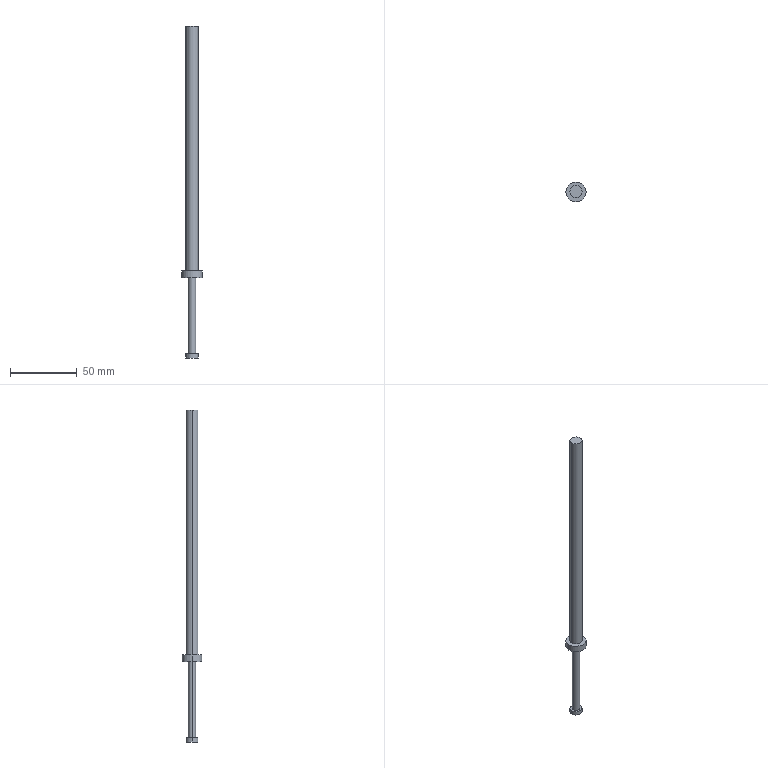Part | Creo | 1 solid | 13 faces | box 15 x 15 x 248 mm | volume 14071 mm3 | cylinder 8 | plane 5 | commonest cylinder face diameters 9 x4 5.5 x2 15 x2
STEP:
#1=CARTESIAN_POINT('',(-188.734,-198.792,-47.5));
#2=VERTEX_POINT('',#1);
#3=CARTESIAN_POINT('',(-179.734,-198.792,-47.5));
#4=VERTEX_POINT('',#3);
#5=CARTESIAN_POINT('',(-184.234,-198.792,-47.5));
#6=DIRECTION('',(0.,0.,1.));
#7=DIRECTION('',(-1.,0.,0.));
#8=AXIS2_PLACEMENT_3D('',#5,#6,#7);
#9=CIRCLE('',#8,4.5);
#10=EDGE_CURVE('',#2,#4,#9,.T.);
#11=ORIENTED_EDGE('',*,*,#10,.T.);
#12=CARTESIAN_POINT('',(-179.734,-198.792,-230.5));
#13=VERTEX_POINT('',#12);
#14=CARTESIAN_POINT('',(-179.734,-198.792,-47.5));
#15=DIRECTION('',(0.,0.,-1.));
#16=VECTOR('',#15,183.);
#17=LINE('',#14,#16);
#18=EDGE_CURVE('',#4,#13,#17,.T.);
#19=ORIENTED_EDGE('',*,*,#18,.T.);
#20=CARTESIAN_POINT('',(-188.734,-198.792,-230.5));
#21=VERTEX_POINT('',#20);
#22=CARTESIAN_POINT('',(-184.234,-198.792,-230.5));
#23=DIRECTION('',(0.,0.,-1.));
#24=DIRECTION('',(1.,0.,0.));
#25=AXIS2_PLACEMENT_3D('',#22,#23,#24);
#26=CIRCLE('',#25,4.5);
#27=EDGE_CURVE('',#13,#21,#26,.T.);
#28=ORIENTED_EDGE('',*,*,#27,.T.);
#29=CARTESIAN_POINT('',(-188.734,-198.792,-47.5));
#30=DIRECTION('',(0.,0.,-1.));
#31=VECTOR('',#30,183.);
#32=LINE('',#29,#31);
#33=EDGE_CURVE('',#2,#21,#32,.T.);
#34=ORIENTED_EDGE('',*,*,#33,.F.);
#35=EDGE_LOOP('',(#11,#19,#28,#34));
#36=FACE_OUTER_BOUND('',#35,.F.);
#37=CARTESIAN_POINT('',(-184.234,-198.792,7.391));
#38=DIRECTION('',(0.,0.,-1.));
#39=DIRECTION('',(1.,0.,0.));
#40=AXIS2_PLACEMENT_3D('',#37,#38,#39);
#41=CYLINDRICAL_SURFACE('',#40,4.5);
#42=ADVANCED_FACE('',(#36),#41,.T.);
#43=ORIENTED_EDGE('',*,*,#10,.F.);
#44=CARTESIAN_POINT('',(-184.234,-198.792,-47.5));
#45=DIRECTION('',(0.,0.,1.));
#46=DIRECTION('',(1.,0.,0.));
#47=AXIS2_PLACEMENT_3D('',#44,#45,#46);
#48=CIRCLE('',#47,4.5);
#49=EDGE_CURVE('',#4,#2,#48,.T.);
#50=ORIENTED_EDGE('',*,*,#49,.F.);
#51=EDGE_LOOP('',(#43,#50));
#52=FACE_OUTER_BOUND('',#51,.F.);
#53=CARTESIAN_POINT('',(0.,0.,-47.5));
#54=DIRECTION('',(0.,0.,-1.));
#55=DIRECTION('',(-1.,0.,0.));
#56=AXIS2_PLACEMENT_3D('',#53,#54,#55);
#57=PLANE('',#56);
#58=ADVANCED_FACE('',(#52),#57,.F.);
#59=ORIENTED_EDGE('',*,*,#49,.T.);
#60=ORIENTED_EDGE('',*,*,#33,.T.);
#61=CARTESIAN_POINT('',(-184.234,-198.792,-230.5));
#62=DIRECTION('',(0.,0.,-1.));
#63=DIRECTION('',(-1.,0.,0.));
#64=AXIS2_PLACEMENT_3D('',#61,#62,#63);
#65=CIRCLE('',#64,4.5);
#66=EDGE_CURVE('',#21,#13,#65,.T.);
#67=ORIENTED_EDGE('',*,*,#66,.T.);
#68=ORIENTED_EDGE('',*,*,#18,.F.);
#69=EDGE_LOOP('',(#59,#60,#67,#68));
#70=FACE_OUTER_BOUND('',#69,.F.);
#71=CARTESIAN_POINT('',(-184.234,-198.792,7.391));
#72=DIRECTION('',(0.,0.,-1.));
#73=DIRECTION('',(1.,0.,0.));
#74=AXIS2_PLACEMENT_3D('',#71,#72,#73);
#75=CYLINDRICAL_SURFACE('',#74,4.5);
#76=ADVANCED_FACE('',(#70),#75,.T.);
#77=CARTESIAN_POINT('',(-176.734,-198.792,-230.5));
#78=VERTEX_POINT('',#77);
#79=CARTESIAN_POINT('',(-191.734,-198.792,-230.5));
#80=VERTEX_POINT('',#79);
#81=CARTESIAN_POINT('',(-184.234,-198.792,-230.5));
#82=DIRECTION('',(0.,0.,1.));
#83=DIRECTION('',(1.,0.,0.));
#84=AXIS2_PLACEMENT_3D('',#81,#82,#83);
#85=CIRCLE('',#84,7.5);
#86=EDGE_CURVE('',#78,#80,#85,.T.);
#87=ORIENTED_EDGE('',*,*,#86,.F.);
#88=CARTESIAN_POINT('',(-184.234,-198.792,-230.5));
#89=DIRECTION('',(0.,0.,1.));
#90=DIRECTION('',(-1.,0.,0.));
#91=AXIS2_PLACEMENT_3D('',#88,#89,#90);
#92=CIRCLE('',#91,7.5);
#93=EDGE_CURVE('',#80,#78,#92,.T.);
#94=ORIENTED_EDGE('',*,*,#93,.F.);
#95=EDGE_LOOP('',(#87,#94));
#96=FACE_OUTER_BOUND('',#95,.F.);
#97=ORIENTED_EDGE('',*,*,#27,.F.);
#98=ORIENTED_EDGE('',*,*,#66,.F.);
#99=EDGE_LOOP('',(#97,#98));
#100=FACE_BOUND('',#99,.F.);
#101=CARTESIAN_POINT('',(-184.234,-198.792,-230.5));
#102=DIRECTION('',(0.,0.,1.));
#103=DIRECTION('',(-1.,0.,0.));
#104=AXIS2_PLACEMENT_3D('',#101,#102,#103);
#105=PLANE('',#104);
#106=ADVANCED_FACE('',(#96,#100),#105,.T.);
#107=ORIENTED_EDGE('',*,*,#86,.T.);
#108=CARTESIAN_POINT('',(-191.734,-198.792,-235.5));
#109=VERTEX_POINT('',#108);
#110=CARTESIAN_POINT('',(-191.734,-198.792,-235.5));
#111=DIRECTION('',(0.,0.,1.));
#112=VECTOR('',#111,5.);
#113=LINE('',#110,#112);
#114=EDGE_CURVE('',#109,#80,#113,.T.);
#115=ORIENTED_EDGE('',*,*,#114,.F.);
#116=CARTESIAN_POINT('',(-176.734,-198.792,-235.5));
#117=VERTEX_POINT('',#116);
#118=CARTESIAN_POINT('',(-184.234,-198.792,-235.5));
#119=DIRECTION('',(0.,0.,-1.));
#120=DIRECTION('',(-1.,0.,0.));
#121=AXIS2_PLACEMENT_3D('',#118,#119,#120);
#122=CIRCLE('',#121,7.5);
#123=EDGE_CURVE('',#109,#117,#122,.T.);
#124=ORIENTED_EDGE('',*,*,#123,.T.);
#125=CARTESIAN_POINT('',(-176.734,-198.792,-235.5));
#126=DIRECTION('',(0.,0.,1.));
#127=VECTOR('',#126,5.);
#128=LINE('',#125,#127);
#129=EDGE_CURVE('',#117,#78,#128,.T.);
#130=ORIENTED_EDGE('',*,*,#129,.T.);
#131=EDGE_LOOP('',(#107,#115,#124,#130));
#132=FACE_OUTER_BOUND('',#131,.F.);
#133=CARTESIAN_POINT('',(-184.234,-198.792,-235.5));
#134=DIRECTION('',(0.,0.,1.));
#135=DIRECTION('',(-1.,0.,0.));
#136=AXIS2_PLACEMENT_3D('',#133,#134,#135);
#137=CYLINDRICAL_SURFACE('',#136,7.5);
#138=ADVANCED_FACE('',(#132),#137,.T.);
#139=ORIENTED_EDGE('',*,*,#93,.T.);
#140=ORIENTED_EDGE('',*,*,#129,.F.);
#141=CARTESIAN_POINT('',(-184.234,-198.792,-235.5));
#142=DIRECTION('',(0.,0.,-1.));
#143=DIRECTION('',(1.,0.,0.));
#144=AXIS2_PLACEMENT_3D('',#141,#142,#143);
#145=CIRCLE('',#144,7.5);
#146=EDGE_CURVE('',#117,#109,#145,.T.);
#147=ORIENTED_EDGE('',*,*,#146,.T.);
#148=ORIENTED_EDGE('',*,*,#114,.T.);
#149=EDGE_LOOP('',(#139,#140,#147,#148));
#150=FACE_OUTER_BOUND('',#149,.F.);
#151=CARTESIAN_POINT('',(-184.234,-198.792,-235.5));
#152=DIRECTION('',(0.,0.,1.));
#153=DIRECTION('',(-1.,0.,0.));
#154=AXIS2_PLACEMENT_3D('',#151,#152,#153);
#155=CYLINDRICAL_SURFACE('',#154,7.5);
#156=ADVANCED_FACE('',(#150),#155,.T.);
#157=ORIENTED_EDGE('',*,*,#123,.F.);
#158=ORIENTED_EDGE('',*,*,#146,.F.);
#159=EDGE_LOOP('',(#157,#158));
#160=FACE_OUTER_BOUND('',#159,.F.);
#161=CARTESIAN_POINT('',(-181.484,-198.792,-235.5));
#162=VERTEX_POINT('',#161);
#163=CARTESIAN_POINT('',(-186.984,-198.792,-235.5));
#164=VERTEX_POINT('',#163);
#165=CARTESIAN_POINT('',(-184.234,-198.792,-235.5));
#166=DIRECTION('',(0.,0.,1.));
#167=DIRECTION('',(1.,0.,0.));
#168=AXIS2_PLACEMENT_3D('',#165,#166,#167);
#169=CIRCLE('',#168,2.75);
#170=EDGE_CURVE('',#162,#164,#169,.T.);
#171=ORIENTED_EDGE('',*,*,#170,.F.);
#172=CARTESIAN_POINT('',(-184.234,-198.792,-235.5));
#173=DIRECTION('',(0.,0.,1.));
#174=DIRECTION('',(-1.,0.,0.));
#175=AXIS2_PLACEMENT_3D('',#172,#173,#174);
#176=CIRCLE('',#175,2.75);
#177=EDGE_CURVE('',#164,#162,#176,.T.);
#178=ORIENTED_EDGE('',*,*,#177,.F.);
#179=EDGE_LOOP('',(#171,#178));
#180=FACE_BOUND('',#179,.F.);
#181=CARTESIAN_POINT('',(-246.549,-835.47,-235.5));
#182=DIRECTION('',(0.,0.,-1.));
#183=DIRECTION('',(1.,0.,0.));
#184=AXIS2_PLACEMENT_3D('',#181,#182,#183);
#185=PLANE('',#184);
#186=ADVANCED_FACE('',(#160,#180),#185,.T.);
#187=ORIENTED_EDGE('',*,*,#170,.T.);
#188=CARTESIAN_POINT('',(-186.984,-198.792,-292.5));
#189=VERTEX_POINT('',#188);
#190=CARTESIAN_POINT('',(-186.984,-198.792,-235.5));
#191=DIRECTION('',(0.,0.,-1.));
#192=VECTOR('',#191,57.);
#193=LINE('',#190,#192);
#194=EDGE_CURVE('',#164,#189,#193,.T.);
#195=ORIENTED_EDGE('',*,*,#194,.T.);
#196=CARTESIAN_POINT('',(-181.484,-198.792,-292.5));
#197=VERTEX_POINT('',#196);
#198=CARTESIAN_POINT('',(-184.234,-198.792,-292.5));
#199=DIRECTION('',(0.,0.,-1.));
#200=DIRECTION('',(-1.,0.,0.));
#201=AXIS2_PLACEMENT_3D('',#198,#199,#200);
#202=CIRCLE('',#201,2.75);
#203=EDGE_CURVE('',#189,#197,#202,.T.);
#204=ORIENTED_EDGE('',*,*,#203,.T.);
#205=CARTESIAN_POINT('',(-181.484,-198.792,-235.5));
#206=DIRECTION('',(0.,0.,-1.));
#207=VECTOR('',#206,57.);
#208=LINE('',#205,#207);
#209=EDGE_CURVE('',#162,#197,#208,.T.);
#210=ORIENTED_EDGE('',*,*,#209,.F.);
#211=EDGE_LOOP('',(#187,#195,#204,#210));
#212=FACE_OUTER_BOUND('',#211,.F.);
#213=CARTESIAN_POINT('',(-184.234,-198.792,7.391));
#214=DIRECTION('',(0.,0.,-1.));
#215=DIRECTION('',(1.,0.,0.));
#216=AXIS2_PLACEMENT_3D('',#213,#214,#215);
#217=CYLINDRICAL_SURFACE('',#216,2.75);
#218=ADVANCED_FACE('',(#212),#217,.T.);
#219=ORIENTED_EDGE('',*,*,#177,.T.);
#220=ORIENTED_EDGE('',*,*,#209,.T.);
#221=CARTESIAN_POINT('',(-184.234,-198.792,-292.5));
#222=DIRECTION('',(0.,0.,-1.));
#223=DIRECTION('',(1.,0.,0.));
#224=AXIS2_PLACEMENT_3D('',#221,#222,#223);
#225=CIRCLE('',#224,2.75);
#226=EDGE_CURVE('',#197,#189,#225,.T.);
#227=ORIENTED_EDGE('',*,*,#226,.T.);
#228=ORIENTED_EDGE('',*,*,#194,.F.);
#229=EDGE_LOOP('',(#219,#220,#227,#228));
#230=FACE_OUTER_BOUND('',#229,.F.);
#231=CARTESIAN_POINT('',(-184.234,-198.792,7.391));
#232=DIRECTION('',(0.,0.,-1.));
#233=DIRECTION('',(1.,0.,0.));
#234=AXIS2_PLACEMENT_3D('',#231,#232,#233);
#235=CYLINDRICAL_SURFACE('',#234,2.75);
#236=ADVANCED_FACE('',(#230),#235,.T.);
#237=CARTESIAN_POINT('',(-188.734,-198.792,-292.5));
#238=VERTEX_POINT('',#237);
#239=CARTESIAN_POINT('',(-179.734,-198.792,-292.5));
#240=VERTEX_POINT('',#239);
#241=CARTESIAN_POINT('',(-184.234,-198.792,-292.5));
#242=DIRECTION('',(0.,0.,1.));
#243=DIRECTION('',(-1.,0.,0.));
#244=AXIS2_PLACEMENT_3D('',#241,#242,#243);
#245=CIRCLE('',#244,4.5);
#246=EDGE_CURVE('',#238,#240,#245,.T.);
#247=ORIENTED_EDGE('',*,*,#246,.F.);
#248=CARTESIAN_POINT('',(-184.234,-198.792,-292.5));
#249=DIRECTION('',(0.,0.,1.));
#250=DIRECTION('',(1.,0.,0.));
#251=AXIS2_PLACEMENT_3D('',#248,#249,#250);
#252=CIRCLE('',#251,4.5);
#253=EDGE_CURVE('',#240,#238,#252,.T.);
#254=ORIENTED_EDGE('',*,*,#253,.F.);
#255=EDGE_LOOP('',(#247,#254));
#256=FACE_OUTER_BOUND('',#255,.F.);
#257=ORIENTED_EDGE('',*,*,#203,.F.);
#258=ORIENTED_EDGE('',*,*,#226,.F.);
#259=EDGE_LOOP('',(#257,#258));
#260=FACE_BOUND('',#259,.F.);
#261=CARTESIAN_POINT('',(-184.234,-198.792,-292.5));
#262=DIRECTION('',(0.,0.,1.));
#263=DIRECTION('',(-1.,0.,0.));
#264=AXIS2_PLACEMENT_3D('',#261,#262,#263);
#265=PLANE('',#264);
#266=ADVANCED_FACE('',(#256,#260),#265,.T.);
#267=ORIENTED_EDGE('',*,*,#246,.T.);
#268=CARTESIAN_POINT('',(-179.734,-198.792,-295.5));
#269=VERTEX_POINT('',#268);
#270=CARTESIAN_POINT('',(-179.734,-198.792,-295.5));
#271=DIRECTION('',(0.,0.,1.));
#272=VECTOR('',#271,3.);
#273=LINE('',#270,#272);
#274=EDGE_CURVE('',#269,#240,#273,.T.);
#275=ORIENTED_EDGE('',*,*,#274,.F.);
#276=CARTESIAN_POINT('',(-188.734,-198.792,-295.5));
#277=VERTEX_POINT('',#276);
#278=CARTESIAN_POINT('',(-184.234,-198.792,-295.5));
#279=DIRECTION('',(0.,0.,-1.));
#280=DIRECTION('',(1.,0.,0.));
#281=AXIS2_PLACEMENT_3D('',#278,#279,#280);
#282=CIRCLE('',#281,4.5);
#283=EDGE_CURVE('',#269,#277,#282,.T.);
#284=ORIENTED_EDGE('',*,*,#283,.T.);
#285=CARTESIAN_POINT('',(-188.734,-198.792,-295.5));
#286=DIRECTION('',(0.,0.,1.));
#287=VECTOR('',#286,3.);
#288=LINE('',#285,#287);
#289=EDGE_CURVE('',#277,#238,#288,.T.);
#290=ORIENTED_EDGE('',*,*,#289,.T.);
#291=EDGE_LOOP('',(#267,#275,#284,#290));
#292=FACE_OUTER_BOUND('',#291,.F.);
#293=CARTESIAN_POINT('',(-184.234,-198.792,-295.5));
#294=DIRECTION('',(0.,0.,1.));
#295=DIRECTION('',(-1.,0.,0.));
#296=AXIS2_PLACEMENT_3D('',#293,#294,#295);
#297=CYLINDRICAL_SURFACE('',#296,4.5);
#298=ADVANCED_FACE('',(#292),#297,.T.);
#299=ORIENTED_EDGE('',*,*,#253,.T.);
#300=ORIENTED_EDGE('',*,*,#289,.F.);
#301=CARTESIAN_POINT('',(-184.234,-198.792,-295.5));
#302=DIRECTION('',(0.,0.,-1.));
#303=DIRECTION('',(-1.,0.,0.));
#304=AXIS2_PLACEMENT_3D('',#301,#302,#303);
#305=CIRCLE('',#304,4.5);
#306=EDGE_CURVE('',#277,#269,#305,.T.);
#307=ORIENTED_EDGE('',*,*,#306,.T.);
#308=ORIENTED_EDGE('',*,*,#274,.T.);
#309=EDGE_LOOP('',(#299,#300,#307,#308));
#310=FACE_OUTER_BOUND('',#309,.F.);
#311=CARTESIAN_POINT('',(-184.234,-198.792,-295.5));
#312=DIRECTION('',(0.,0.,1.));
#313=DIRECTION('',(-1.,0.,0.));
#314=AXIS2_PLACEMENT_3D('',#311,#312,#313);
#315=CYLINDRICAL_SURFACE('',#314,4.5);
#316=ADVANCED_FACE('',(#310),#315,.T.);
#317=ORIENTED_EDGE('',*,*,#283,.F.);
#318=ORIENTED_EDGE('',*,*,#306,.F.);
#319=EDGE_LOOP('',(#317,#318));
#320=FACE_OUTER_BOUND('',#319,.F.);
#321=CARTESIAN_POINT('',(328.451,-835.47,-295.5));
#322=DIRECTION('',(0.,0.,-1.));
#323=DIRECTION('',(1.,0.,0.));
#324=AXIS2_PLACEMENT_3D('',#321,#322,#323);
#325=PLANE('',#324);
#326=ADVANCED_FACE('',(#320),#325,.T.);
#327=CLOSED_SHELL('',(#42,#58,#76,#106,#138,#156,#186,#218,#236,#266,#298,#316,#326));
#328=MANIFOLD_SOLID_BREP('',#327);
#329=(LENGTH_UNIT()NAMED_UNIT(*)SI_UNIT(.MILLI.,.METRE.));
#330=UNCERTAINTY_MEASURE_WITH_UNIT(LENGTH_MEASURE(0.02489),#329,'','');
#331=(NAMED_UNIT(*)PLANE_ANGLE_UNIT()SI_UNIT($,.RADIAN.));
#332=PLANE_ANGLE_MEASURE_WITH_UNIT(PLANE_ANGLE_MEASURE(0.01745),#331);
#333=(CONVERSION_BASED_UNIT('DEGREE',#332)NAMED_UNIT(*)PLANE_ANGLE_UNIT());
#334=(NAMED_UNIT(*)SI_UNIT($,.STERADIAN.)SOLID_ANGLE_UNIT());
#335=(GEOMETRIC_REPRESENTATION_CONTEXT(3)GLOBAL_UNCERTAINTY_ASSIGNED_CONTEXT((#330))GLOBAL_UNIT_ASSIGNED_CONTEXT((#329,#333,#334))REPRESENTATION_CONTEXT('',''));
#336=ADVANCED_BREP_SHAPE_REPRESENTATION('',(#328),#335);